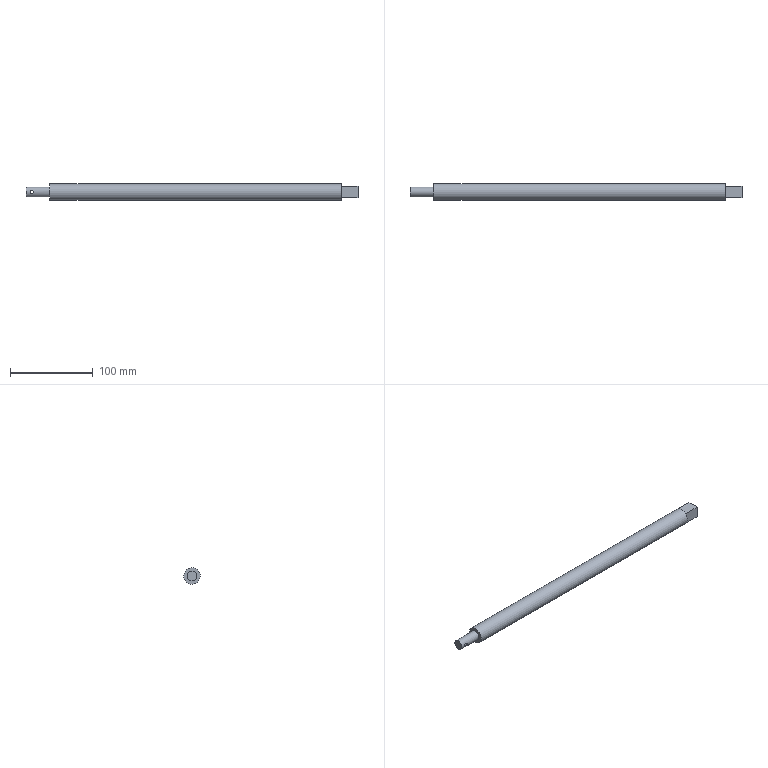Part | STEP file | SN10_001_005_FUSO | 1 solid | 11 faces | box 402 x 20 x 20 mm | volume 117949 mm3 | plane 8 | cylinder 3 | commonest cylinder face diameters 4 x1 12 x1 20 x1
STEP:
#1=CARTESIAN_POINT('',(0.,0.,0.));
#2=DIRECTION('',(0.,0.,1.));
#3=DIRECTION('',(1.,0.,0.));
#4=AXIS2_PLACEMENT_3D('',#1,#2,#3);
#5=CARTESIAN_POINT('',(67.,216.956,-8.776));
#6=VERTEX_POINT('',#5);
#7=CARTESIAN_POINT('',(67.,221.75,0.));
#8=DIRECTION('',(-1.,0.,0.));
#9=DIRECTION('',(0.,1.,0.));
#10=AXIS2_PLACEMENT_3D('',#7,#8,#9);
#11=CIRCLE('',#10,10.);
#12=CARTESIAN_POINT('',(239.,221.75,0.));
#13=DIRECTION('',(-1.,0.,0.));
#14=DIRECTION('',(0.,0.4794,0.8776));
#15=AXIS2_PLACEMENT_3D('',#12,#13,#14);
#16=CYLINDRICAL_SURFACE('',#15,10.);
#17=CARTESIAN_POINT('',(1.071,172.));
#18=DIRECTION('',(1.,0.));
#19=VECTOR('',#18,1.);
#20=LINE('',#17,#19);
#21=(GEOMETRIC_REPRESENTATION_CONTEXT(2)PARAMETRIC_REPRESENTATION_CONTEXT()REPRESENTATION_CONTEXT('',''));
#22=DEFINITIONAL_REPRESENTATION('',(#20),#21);
#23=PCURVE('',#16,#22);
#24=CARTESIAN_POINT('',(67.,221.75,6.));
#25=DIRECTION('',(-1.,0.,0.));
#26=DIRECTION('',(0.,0.,1.));
#27=AXIS2_PLACEMENT_3D('',#24,#25,#26);
#28=PLANE('',#27);
#29=CARTESIAN_POINT('',(-6.,0.));
#30=DIRECTION('',(0.,1.));
#31=AXIS2_PLACEMENT_2D('',#29,#30);
#32=CIRCLE('',#31,10.);
#33=(GEOMETRIC_REPRESENTATION_CONTEXT(2)PARAMETRIC_REPRESENTATION_CONTEXT()REPRESENTATION_CONTEXT('',''));
#34=DEFINITIONAL_REPRESENTATION('',(#32),#33);
#35=PCURVE('',#28,#34);
#36=SURFACE_CURVE('',#11,(#23,#35),.PCURVE_S1.);
#37=EDGE_CURVE('',#6,#6,#36,.T.);
#38=ORIENTED_EDGE('',*,*,#37,.F.);
#39=CARTESIAN_POINT('',(420.,216.956,-8.776));
#40=VERTEX_POINT('',#39);
#41=CARTESIAN_POINT('',(420.,216.956,-8.776));
#42=CARTESIAN_POINT('',(67.,216.956,-8.776));
#43=B_SPLINE_CURVE_WITH_KNOTS('',1,(#41,#42),.UNSPECIFIED.,.F.,.F.,(2,2),(-181.,172.),.PIECEWISE_BEZIER_KNOTS.);
#44=CARTESIAN_POINT('',(3.142,0.));
#45=DIRECTION('',(0.,1.));
#46=VECTOR('',#45,1.);
#47=LINE('',#44,#46);
#48=(GEOMETRIC_REPRESENTATION_CONTEXT(2)PARAMETRIC_REPRESENTATION_CONTEXT()REPRESENTATION_CONTEXT('',''));
#49=DEFINITIONAL_REPRESENTATION('',(#47),#48);
#50=PCURVE('',#16,#49);
#51=CARTESIAN_POINT('',(9.425,0.));
#52=DIRECTION('',(0.,1.));
#53=VECTOR('',#52,1.);
#54=LINE('',#51,#53);
#55=(GEOMETRIC_REPRESENTATION_CONTEXT(2)PARAMETRIC_REPRESENTATION_CONTEXT()REPRESENTATION_CONTEXT('',''));
#56=DEFINITIONAL_REPRESENTATION('',(#54),#55);
#57=PCURVE('',#16,#56);
#58=SEAM_CURVE('',#43,(#50,#57),.PCURVE_S1.);
#59=EDGE_CURVE('',#40,#6,#58,.T.);
#60=ORIENTED_EDGE('',*,*,#59,.F.);
#61=CARTESIAN_POINT('',(420.,221.75,0.));
#62=DIRECTION('',(-1.,0.,0.));
#63=DIRECTION('',(0.,1.,0.));
#64=AXIS2_PLACEMENT_3D('',#61,#62,#63);
#65=CIRCLE('',#64,10.);
#66=CARTESIAN_POINT('',(1.071,-181.));
#67=DIRECTION('',(1.,0.));
#68=VECTOR('',#67,1.);
#69=LINE('',#66,#68);
#70=(GEOMETRIC_REPRESENTATION_CONTEXT(2)PARAMETRIC_REPRESENTATION_CONTEXT()REPRESENTATION_CONTEXT('',''));
#71=DEFINITIONAL_REPRESENTATION('',(#69),#70);
#72=PCURVE('',#16,#71);
#73=CARTESIAN_POINT('',(420.,221.75,10.));
#74=DIRECTION('',(-1.,0.,0.));
#75=DIRECTION('',(0.,0.,1.));
#76=AXIS2_PLACEMENT_3D('',#73,#74,#75);
#77=PLANE('',#76);
#78=CARTESIAN_POINT('',(-10.,0.));
#79=DIRECTION('',(0.,1.));
#80=AXIS2_PLACEMENT_2D('',#78,#79);
#81=CIRCLE('',#80,10.);
#82=(GEOMETRIC_REPRESENTATION_CONTEXT(2)PARAMETRIC_REPRESENTATION_CONTEXT()REPRESENTATION_CONTEXT('',''));
#83=DEFINITIONAL_REPRESENTATION('',(#81),#82);
#84=PCURVE('',#77,#83);
#85=SURFACE_CURVE('',#65,(#72,#84),.PCURVE_S1.);
#86=EDGE_CURVE('',#40,#40,#85,.T.);
#87=ORIENTED_EDGE('',*,*,#86,.T.);
#88=ORIENTED_EDGE('',*,*,#59,.T.);
#89=EDGE_LOOP('',(#38,#60,#87,#88));
#90=FACE_BOUND('',#89,.T.);
#91=ADVANCED_FACE('',(#90),#16,.T.);
#92=CARTESIAN_POINT('',(38.,224.627,5.265));
#93=VERTEX_POINT('',#92);
#94=CARTESIAN_POINT('',(38.,221.75,0.));
#95=DIRECTION('',(-1.,0.,0.));
#96=DIRECTION('',(0.,1.,0.));
#97=AXIS2_PLACEMENT_3D('',#94,#95,#96);
#98=CIRCLE('',#97,6.);
#99=CARTESIAN_POINT('',(38.,221.75,0.));
#100=DIRECTION('',(-1.,0.,0.));
#101=DIRECTION('',(0.,0.,1.));
#102=AXIS2_PLACEMENT_3D('',#99,#100,#101);
#103=PLANE('',#102);
#104=CARTESIAN_POINT('',(0.,0.));
#105=DIRECTION('',(0.,1.));
#106=AXIS2_PLACEMENT_2D('',#104,#105);
#107=CIRCLE('',#106,6.);
#108=(GEOMETRIC_REPRESENTATION_CONTEXT(2)PARAMETRIC_REPRESENTATION_CONTEXT()REPRESENTATION_CONTEXT('',''));
#109=DEFINITIONAL_REPRESENTATION('',(#107),#108);
#110=PCURVE('',#103,#109);
#111=CARTESIAN_POINT('',(239.,221.75,0.));
#112=DIRECTION('',(-1.,0.,0.));
#113=DIRECTION('',(0.,0.4794,0.8776));
#114=AXIS2_PLACEMENT_3D('',#111,#112,#113);
#115=CYLINDRICAL_SURFACE('',#114,6.);
#116=CARTESIAN_POINT('',(-5.212,201.));
#117=DIRECTION('',(1.,0.));
#118=VECTOR('',#117,1.);
#119=LINE('',#116,#118);
#120=(GEOMETRIC_REPRESENTATION_CONTEXT(2)PARAMETRIC_REPRESENTATION_CONTEXT()REPRESENTATION_CONTEXT('',''));
#121=DEFINITIONAL_REPRESENTATION('',(#119),#120);
#122=PCURVE('',#115,#121);
#123=SURFACE_CURVE('',#98,(#110,#122),.PCURVE_S1.);
#124=EDGE_CURVE('',#93,#93,#123,.T.);
#125=ORIENTED_EDGE('',*,*,#124,.T.);
#126=EDGE_LOOP('',(#125));
#127=FACE_BOUND('',#126,.T.);
#128=ADVANCED_FACE('',(#127),#103,.T.);
#129=ORIENTED_EDGE('',*,*,#37,.T.);
#130=EDGE_LOOP('',(#129));
#131=FACE_BOUND('',#130,.T.);
#132=CARTESIAN_POINT('',(67.,224.627,5.265));
#133=VERTEX_POINT('',#132);
#134=CARTESIAN_POINT('',(67.,221.75,0.));
#135=DIRECTION('',(-1.,0.,0.));
#136=DIRECTION('',(0.,1.,0.));
#137=AXIS2_PLACEMENT_3D('',#134,#135,#136);
#138=CIRCLE('',#137,6.);
#139=CARTESIAN_POINT('',(-6.,0.));
#140=DIRECTION('',(0.,1.));
#141=AXIS2_PLACEMENT_2D('',#139,#140);
#142=CIRCLE('',#141,6.);
#143=(GEOMETRIC_REPRESENTATION_CONTEXT(2)PARAMETRIC_REPRESENTATION_CONTEXT()REPRESENTATION_CONTEXT('',''));
#144=DEFINITIONAL_REPRESENTATION('',(#142),#143);
#145=PCURVE('',#28,#144);
#146=CARTESIAN_POINT('',(-5.212,172.));
#147=DIRECTION('',(1.,0.));
#148=VECTOR('',#147,1.);
#149=LINE('',#146,#148);
#150=(GEOMETRIC_REPRESENTATION_CONTEXT(2)PARAMETRIC_REPRESENTATION_CONTEXT()REPRESENTATION_CONTEXT('',''));
#151=DEFINITIONAL_REPRESENTATION('',(#149),#150);
#152=PCURVE('',#115,#151);
#153=SURFACE_CURVE('',#138,(#145,#152),.PCURVE_S1.);
#154=EDGE_CURVE('',#133,#133,#153,.T.);
#155=ORIENTED_EDGE('',*,*,#154,.F.);
#156=EDGE_LOOP('',(#155));
#157=FACE_BOUND('',#156,.T.);
#158=ADVANCED_FACE('',(#131,#157),#28,.T.);
#159=ORIENTED_EDGE('',*,*,#124,.F.);
#160=CARTESIAN_POINT('',(67.,224.627,5.265));
#161=CARTESIAN_POINT('',(38.,224.627,5.265));
#162=B_SPLINE_CURVE_WITH_KNOTS('',1,(#160,#161),.UNSPECIFIED.,.F.,.F.,(2,2),(172.,201.),.PIECEWISE_BEZIER_KNOTS.);
#163=CARTESIAN_POINT('',(0.,0.));
#164=DIRECTION('',(0.,1.));
#165=VECTOR('',#164,1.);
#166=LINE('',#163,#165);
#167=(GEOMETRIC_REPRESENTATION_CONTEXT(2)PARAMETRIC_REPRESENTATION_CONTEXT()REPRESENTATION_CONTEXT('',''));
#168=DEFINITIONAL_REPRESENTATION('',(#166),#167);
#169=PCURVE('',#115,#168);
#170=CARTESIAN_POINT('',(6.283,0.));
#171=DIRECTION('',(0.,1.));
#172=VECTOR('',#171,1.);
#173=LINE('',#170,#172);
#174=(GEOMETRIC_REPRESENTATION_CONTEXT(2)PARAMETRIC_REPRESENTATION_CONTEXT()REPRESENTATION_CONTEXT('',''));
#175=DEFINITIONAL_REPRESENTATION('',(#173),#174);
#176=PCURVE('',#115,#175);
#177=SEAM_CURVE('',#162,(#169,#176),.PCURVE_S1.);
#178=EDGE_CURVE('',#133,#93,#177,.T.);
#179=ORIENTED_EDGE('',*,*,#178,.F.);
#180=ORIENTED_EDGE('',*,*,#154,.T.);
#181=ORIENTED_EDGE('',*,*,#178,.T.);
#182=EDGE_LOOP('',(#159,#179,#180,#181));
#183=FACE_BOUND('',#182,.T.);
#184=CARTESIAN_POINT('',(45.,227.407,2.));
#185=VERTEX_POINT('',#184);
#186=CARTESIAN_POINT('',(45.,227.407,-2.));
#187=VERTEX_POINT('',#186);
#188=CARTESIAN_POINT('',(45.,227.407,2.));
#189=CARTESIAN_POINT('',(45.253,227.407,2.));
#190=CARTESIAN_POINT('',(45.522,227.426,1.949));
#191=CARTESIAN_POINT('',(46.014,227.492,1.744));
#192=CARTESIAN_POINT('',(46.238,227.538,1.591));
#193=CARTESIAN_POINT('',(46.591,227.624,1.238));
#194=CARTESIAN_POINT('',(46.744,227.669,1.014));
#195=CARTESIAN_POINT('',(46.949,227.732,0.5219));
#196=CARTESIAN_POINT('',(47.,227.75,0.2532));
#197=CARTESIAN_POINT('',(47.,227.75,-0.2532));
#198=CARTESIAN_POINT('',(46.949,227.732,-0.5219));
#199=CARTESIAN_POINT('',(46.744,227.669,-1.014));
#200=CARTESIAN_POINT('',(46.591,227.624,-1.238));
#201=CARTESIAN_POINT('',(46.238,227.538,-1.591));
#202=CARTESIAN_POINT('',(46.014,227.492,-1.744));
#203=CARTESIAN_POINT('',(45.522,227.426,-1.949));
#204=CARTESIAN_POINT('',(45.253,227.407,-2.));
#205=CARTESIAN_POINT('',(45.,227.407,-2.));
#206=B_SPLINE_CURVE_WITH_KNOTS('',3,(#188,#189,#190,#191,#192,#193,#194,#195,#196,#197,#198,#199,#200,#201,#202,#203,#204,#205),.UNSPECIFIED.,.F.,.F.,(4,2,2,2,2,2,2,2,4),(0.6078,0.6837,0.7597,0.8357,0.9116,0.9876,1.064,1.14,1.216),.UNSPECIFIED.);
#207=CARTESIAN_POINT('',(0.731,194.));
#208=CARTESIAN_POINT('',(0.731,193.954));
#209=CARTESIAN_POINT('',(0.7316,193.861));
#210=CARTESIAN_POINT('',(0.7342,193.72));
#211=CARTESIAN_POINT('',(0.7387,193.578));
#212=CARTESIAN_POINT('',(0.745,193.437));
#213=CARTESIAN_POINT('',(0.753,193.299));
#214=CARTESIAN_POINT('',(0.7628,193.165));
#215=CARTESIAN_POINT('',(0.7742,193.035));
#216=CARTESIAN_POINT('',(0.7871,192.912));
#217=CARTESIAN_POINT('',(0.8013,192.795));
#218=CARTESIAN_POINT('',(0.8166,192.685));
#219=CARTESIAN_POINT('',(0.8326,192.585));
#220=CARTESIAN_POINT('',(0.8498,192.491));
#221=CARTESIAN_POINT('',(0.8685,192.403));
#222=CARTESIAN_POINT('',(0.8883,192.321));
#223=CARTESIAN_POINT('',(0.9093,192.247));
#224=CARTESIAN_POINT('',(0.9311,192.181));
#225=CARTESIAN_POINT('',(0.9537,192.125));
#226=CARTESIAN_POINT('',(0.9768,192.079));
#227=CARTESIAN_POINT('',(1.,192.044));
#228=CARTESIAN_POINT('',(1.024,192.019));
#229=CARTESIAN_POINT('',(1.048,192.003));
#230=CARTESIAN_POINT('',(1.071,191.998));
#231=CARTESIAN_POINT('',(1.094,192.003));
#232=CARTESIAN_POINT('',(1.118,192.019));
#233=CARTESIAN_POINT('',(1.141,192.044));
#234=CARTESIAN_POINT('',(1.165,192.079));
#235=CARTESIAN_POINT('',(1.188,192.125));
#236=CARTESIAN_POINT('',(1.211,192.181));
#237=CARTESIAN_POINT('',(1.232,192.247));
#238=CARTESIAN_POINT('',(1.253,192.321));
#239=CARTESIAN_POINT('',(1.273,192.403));
#240=CARTESIAN_POINT('',(1.292,192.491));
#241=CARTESIAN_POINT('',(1.309,192.585));
#242=CARTESIAN_POINT('',(1.325,192.685));
#243=CARTESIAN_POINT('',(1.34,192.795));
#244=CARTESIAN_POINT('',(1.354,192.912));
#245=CARTESIAN_POINT('',(1.367,193.035));
#246=CARTESIAN_POINT('',(1.379,193.165));
#247=CARTESIAN_POINT('',(1.389,193.299));
#248=CARTESIAN_POINT('',(1.397,193.437));
#249=CARTESIAN_POINT('',(1.403,193.578));
#250=CARTESIAN_POINT('',(1.407,193.72));
#251=CARTESIAN_POINT('',(1.41,193.861));
#252=CARTESIAN_POINT('',(1.411,193.954));
#253=CARTESIAN_POINT('',(1.411,194.));
#254=B_SPLINE_CURVE_WITH_KNOTS('',3,(#207,#208,#209,#210,#211,#212,#213,#214,#215,#216,#217,#218,#219,#220,#221,#222,#223,#224,#225,#226,#227,#228,#229,#230,#231,#232,#233,#234,#235,#236,#237,#238,#239,#240,#241,#242,#243,#244,#245,#246,#247,#248,#249,#250,#251,#252,#253),.UNSPECIFIED.,.F.,.F.,(4,1,1,1,1,1,1,1,1,1,1,1,1,1,1,1,1,1,1,1,1,1,1,1,1,1,1,1,1,1,1,1,1,1,1,1,1,1,1,1,1,1,1,1,4),(0.6078,0.6216,0.6354,0.6492,0.663,0.6768,0.6906,0.7044,0.7183,0.7321,0.7459,0.7597,0.7735,0.7873,0.8011,0.815,0.8288,0.8426,0.8564,0.8702,0.884,0.8978,0.9116,0.9255,0.9393,0.9531,0.9669,0.9807,0.9945,1.008,1.022,1.036,1.05,1.064,1.077,1.091,1.105,1.119,1.133,1.146,1.16,1.174,1.188,1.202,1.216),.QUASI_UNIFORM_KNOTS.);
#255=(GEOMETRIC_REPRESENTATION_CONTEXT(2)PARAMETRIC_REPRESENTATION_CONTEXT()REPRESENTATION_CONTEXT('',''));
#256=DEFINITIONAL_REPRESENTATION('',(#254),#255);
#257=PCURVE('',#115,#256);
#258=CARTESIAN_POINT('',(45.,221.75,0.));
#259=DIRECTION('',(0.,1.,0.));
#260=DIRECTION('',(0.,0.,1.));
#261=AXIS2_PLACEMENT_3D('',#258,#259,#260);
#262=CYLINDRICAL_SURFACE('',#261,2.);
#263=CARTESIAN_POINT('',(0.,5.657));
#264=CARTESIAN_POINT('',(0.02302,5.657));
#265=CARTESIAN_POINT('',(0.06957,5.658));
#266=CARTESIAN_POINT('',(0.1406,5.664));
#267=CARTESIAN_POINT('',(0.2125,5.672));
#268=CARTESIAN_POINT('',(0.285,5.684));
#269=CARTESIAN_POINT('',(0.3577,5.7));
#270=CARTESIAN_POINT('',(0.4304,5.718));
#271=CARTESIAN_POINT('',(0.5029,5.738));
#272=CARTESIAN_POINT('',(0.575,5.76));
#273=CARTESIAN_POINT('',(0.6463,5.784));
#274=CARTESIAN_POINT('',(0.7167,5.807));
#275=CARTESIAN_POINT('',(0.7852,5.831));
#276=CARTESIAN_POINT('',(0.8538,5.854));
#277=CARTESIAN_POINT('',(0.9242,5.878));
#278=CARTESIAN_POINT('',(0.9955,5.901));
#279=CARTESIAN_POINT('',(1.068,5.922));
#280=CARTESIAN_POINT('',(1.14,5.942));
#281=CARTESIAN_POINT('',(1.213,5.959));
#282=CARTESIAN_POINT('',(1.286,5.974));
#283=CARTESIAN_POINT('',(1.358,5.985));
#284=CARTESIAN_POINT('',(1.43,5.994));
#285=CARTESIAN_POINT('',(1.501,5.999));
#286=CARTESIAN_POINT('',(1.571,6.001));
#287=CARTESIAN_POINT('',(1.64,5.999));
#288=CARTESIAN_POINT('',(1.711,5.994));
#289=CARTESIAN_POINT('',(1.783,5.985));
#290=CARTESIAN_POINT('',(1.856,5.974));
#291=CARTESIAN_POINT('',(1.929,5.959));
#292=CARTESIAN_POINT('',(2.001,5.942));
#293=CARTESIAN_POINT('',(2.074,5.922));
#294=CARTESIAN_POINT('',(2.146,5.901));
#295=CARTESIAN_POINT('',(2.217,5.878));
#296=CARTESIAN_POINT('',(2.288,5.854));
#297=CARTESIAN_POINT('',(2.356,5.831));
#298=CARTESIAN_POINT('',(2.425,5.807));
#299=CARTESIAN_POINT('',(2.495,5.784));
#300=CARTESIAN_POINT('',(2.567,5.76));
#301=CARTESIAN_POINT('',(2.639,5.738));
#302=CARTESIAN_POINT('',(2.711,5.718));
#303=CARTESIAN_POINT('',(2.784,5.7));
#304=CARTESIAN_POINT('',(2.857,5.684));
#305=CARTESIAN_POINT('',(2.929,5.672));
#306=CARTESIAN_POINT('',(3.001,5.664));
#307=CARTESIAN_POINT('',(3.072,5.658));
#308=CARTESIAN_POINT('',(3.119,5.657));
#309=CARTESIAN_POINT('',(3.142,5.657));
#310=B_SPLINE_CURVE_WITH_KNOTS('',3,(#263,#264,#265,#266,#267,#268,#269,#270,#271,#272,#273,#274,#275,#276,#277,#278,#279,#280,#281,#282,#283,#284,#285,#286,#287,#288,#289,#290,#291,#292,#293,#294,#295,#296,#297,#298,#299,#300,#301,#302,#303,#304,#305,#306,#307,#308,#309),.UNSPECIFIED.,.F.,.F.,(4,1,1,1,1,1,1,1,1,1,1,1,1,1,1,1,1,1,1,1,1,1,1,1,1,1,1,1,1,1,1,1,1,1,1,1,1,1,1,1,1,1,1,1,4),(0.6078,0.6216,0.6354,0.6492,0.663,0.6768,0.6906,0.7044,0.7183,0.7321,0.7459,0.7597,0.7735,0.7873,0.8011,0.815,0.8288,0.8426,0.8564,0.8702,0.884,0.8978,0.9116,0.9255,0.9393,0.9531,0.9669,0.9807,0.9945,1.008,1.022,1.036,1.05,1.064,1.077,1.091,1.105,1.119,1.133,1.146,1.16,1.174,1.188,1.202,1.216),.QUASI_UNIFORM_KNOTS.);
#311=(GEOMETRIC_REPRESENTATION_CONTEXT(2)PARAMETRIC_REPRESENTATION_CONTEXT()REPRESENTATION_CONTEXT('',''));
#312=DEFINITIONAL_REPRESENTATION('',(#310),#311);
#313=PCURVE('',#262,#312);
#314=SURFACE_CURVE('',#206,(#257,#313),.PCURVE_S1.);
#315=EDGE_CURVE('',#185,#187,#314,.T.);
#316=ORIENTED_EDGE('',*,*,#315,.F.);
#317=CARTESIAN_POINT('',(45.,227.407,-2.));
#318=CARTESIAN_POINT('',(44.747,227.407,-2.));
#319=CARTESIAN_POINT('',(44.478,227.426,-1.949));
#320=CARTESIAN_POINT('',(43.986,227.492,-1.744));
#321=CARTESIAN_POINT('',(43.762,227.538,-1.591));
#322=CARTESIAN_POINT('',(43.409,227.624,-1.238));
#323=CARTESIAN_POINT('',(43.256,227.669,-1.014));
#324=CARTESIAN_POINT('',(43.051,227.732,-0.5219));
#325=CARTESIAN_POINT('',(43.,227.75,-0.2532));
#326=CARTESIAN_POINT('',(43.,227.75,0.2532));
#327=CARTESIAN_POINT('',(43.051,227.732,0.5219));
#328=CARTESIAN_POINT('',(43.256,227.669,1.014));
#329=CARTESIAN_POINT('',(43.409,227.624,1.238));
#330=CARTESIAN_POINT('',(43.762,227.538,1.591));
#331=CARTESIAN_POINT('',(43.986,227.492,1.744));
#332=CARTESIAN_POINT('',(44.478,227.426,1.949));
#333=CARTESIAN_POINT('',(44.747,227.407,2.));
#334=CARTESIAN_POINT('',(45.,227.407,2.));
#335=B_SPLINE_CURVE_WITH_KNOTS('',3,(#317,#318,#319,#320,#321,#322,#323,#324,#325,#326,#327,#328,#329,#330,#331,#332,#333,#334),.UNSPECIFIED.,.F.,.F.,(4,2,2,2,2,2,2,2,4),(0.,0.07599,0.152,0.2279,0.3039,0.3798,0.4558,0.5318,0.6078),.UNSPECIFIED.);
#336=CARTESIAN_POINT('',(1.411,194.));
#337=CARTESIAN_POINT('',(1.411,194.046));
#338=CARTESIAN_POINT('',(1.41,194.139));
#339=CARTESIAN_POINT('',(1.407,194.28));
#340=CARTESIAN_POINT('',(1.403,194.422));
#341=CARTESIAN_POINT('',(1.397,194.563));
#342=CARTESIAN_POINT('',(1.389,194.701));
#343=CARTESIAN_POINT('',(1.379,194.835));
#344=CARTESIAN_POINT('',(1.367,194.965));
#345=CARTESIAN_POINT('',(1.354,195.088));
#346=CARTESIAN_POINT('',(1.34,195.205));
#347=CARTESIAN_POINT('',(1.325,195.315));
#348=CARTESIAN_POINT('',(1.309,195.415));
#349=CARTESIAN_POINT('',(1.292,195.509));
#350=CARTESIAN_POINT('',(1.273,195.597));
#351=CARTESIAN_POINT('',(1.253,195.679));
#352=CARTESIAN_POINT('',(1.232,195.753));
#353=CARTESIAN_POINT('',(1.211,195.819));
#354=CARTESIAN_POINT('',(1.188,195.875));
#355=CARTESIAN_POINT('',(1.165,195.921));
#356=CARTESIAN_POINT('',(1.141,195.956));
#357=CARTESIAN_POINT('',(1.118,195.981));
#358=CARTESIAN_POINT('',(1.094,195.997));
#359=CARTESIAN_POINT('',(1.071,196.002));
#360=CARTESIAN_POINT('',(1.048,195.997));
#361=CARTESIAN_POINT('',(1.024,195.981));
#362=CARTESIAN_POINT('',(1.,195.956));
#363=CARTESIAN_POINT('',(0.9768,195.921));
#364=CARTESIAN_POINT('',(0.9537,195.875));
#365=CARTESIAN_POINT('',(0.9311,195.819));
#366=CARTESIAN_POINT('',(0.9093,195.753));
#367=CARTESIAN_POINT('',(0.8883,195.679));
#368=CARTESIAN_POINT('',(0.8685,195.597));
#369=CARTESIAN_POINT('',(0.8498,195.509));
#370=CARTESIAN_POINT('',(0.8326,195.415));
#371=CARTESIAN_POINT('',(0.8166,195.315));
#372=CARTESIAN_POINT('',(0.8013,195.205));
#373=CARTESIAN_POINT('',(0.7871,195.088));
#374=CARTESIAN_POINT('',(0.7742,194.965));
#375=CARTESIAN_POINT('',(0.7628,194.835));
#376=CARTESIAN_POINT('',(0.753,194.701));
#377=CARTESIAN_POINT('',(0.745,194.563));
#378=CARTESIAN_POINT('',(0.7387,194.422));
#379=CARTESIAN_POINT('',(0.7342,194.28));
#380=CARTESIAN_POINT('',(0.7316,194.139));
#381=CARTESIAN_POINT('',(0.731,194.046));
#382=CARTESIAN_POINT('',(0.731,194.));
#383=B_SPLINE_CURVE_WITH_KNOTS('',3,(#336,#337,#338,#339,#340,#341,#342,#343,#344,#345,#346,#347,#348,#349,#350,#351,#352,#353,#354,#355,#356,#357,#358,#359,#360,#361,#362,#363,#364,#365,#366,#367,#368,#369,#370,#371,#372,#373,#374,#375,#376,#377,#378,#379,#380,#381,#382),.UNSPECIFIED.,.F.,.F.,(4,1,1,1,1,1,1,1,1,1,1,1,1,1,1,1,1,1,1,1,1,1,1,1,1,1,1,1,1,1,1,1,1,1,1,1,1,1,1,1,1,1,1,1,4),(0.,0.01381,0.02763,0.04144,0.05525,0.06906,0.08288,0.09669,0.1105,0.1243,0.1381,0.1519,0.1658,0.1796,0.1934,0.2072,0.221,0.2348,0.2486,0.2624,0.2763,0.2901,0.3039,0.3177,0.3315,0.3453,0.3591,0.3729,0.3868,0.4006,0.4144,0.4282,0.442,0.4558,0.4696,0.4834,0.4973,0.5111,0.5249,0.5387,0.5525,0.5663,0.5801,0.5939,0.6078),.QUASI_UNIFORM_KNOTS.);
#384=(GEOMETRIC_REPRESENTATION_CONTEXT(2)PARAMETRIC_REPRESENTATION_CONTEXT()REPRESENTATION_CONTEXT('',''));
#385=DEFINITIONAL_REPRESENTATION('',(#383),#384);
#386=PCURVE('',#115,#385);
#387=CARTESIAN_POINT('',(3.142,5.657));
#388=CARTESIAN_POINT('',(3.165,5.657));
#389=CARTESIAN_POINT('',(3.211,5.658));
#390=CARTESIAN_POINT('',(3.282,5.664));
#391=CARTESIAN_POINT('',(3.354,5.672));
#392=CARTESIAN_POINT('',(3.427,5.684));
#393=CARTESIAN_POINT('',(3.499,5.7));
#394=CARTESIAN_POINT('',(3.572,5.718));
#395=CARTESIAN_POINT('',(3.644,5.738));
#396=CARTESIAN_POINT('',(3.717,5.76));
#397=CARTESIAN_POINT('',(3.788,5.784));
#398=CARTESIAN_POINT('',(3.858,5.807));
#399=CARTESIAN_POINT('',(3.927,5.831));
#400=CARTESIAN_POINT('',(3.995,5.854));
#401=CARTESIAN_POINT('',(4.066,5.878));
#402=CARTESIAN_POINT('',(4.137,5.901));
#403=CARTESIAN_POINT('',(4.209,5.922));
#404=CARTESIAN_POINT('',(4.282,5.942));
#405=CARTESIAN_POINT('',(4.355,5.959));
#406=CARTESIAN_POINT('',(4.427,5.974));
#407=CARTESIAN_POINT('',(4.5,5.985));
#408=CARTESIAN_POINT('',(4.572,5.994));
#409=CARTESIAN_POINT('',(4.643,5.999));
#410=CARTESIAN_POINT('',(4.712,6.001));
#411=CARTESIAN_POINT('',(4.782,5.999));
#412=CARTESIAN_POINT('',(4.853,5.994));
#413=CARTESIAN_POINT('',(4.925,5.985));
#414=CARTESIAN_POINT('',(4.998,5.974));
#415=CARTESIAN_POINT('',(5.07,5.959));
#416=CARTESIAN_POINT('',(5.143,5.942));
#417=CARTESIAN_POINT('',(5.216,5.922));
#418=CARTESIAN_POINT('',(5.288,5.901));
#419=CARTESIAN_POINT('',(5.359,5.878));
#420=CARTESIAN_POINT('',(5.429,5.854));
#421=CARTESIAN_POINT('',(5.498,5.831));
#422=CARTESIAN_POINT('',(5.567,5.807));
#423=CARTESIAN_POINT('',(5.637,5.784));
#424=CARTESIAN_POINT('',(5.708,5.76));
#425=CARTESIAN_POINT('',(5.78,5.738));
#426=CARTESIAN_POINT('',(5.853,5.718));
#427=CARTESIAN_POINT('',(5.925,5.7));
#428=CARTESIAN_POINT('',(5.998,5.684));
#429=CARTESIAN_POINT('',(6.071,5.672));
#430=CARTESIAN_POINT('',(6.143,5.664));
#431=CARTESIAN_POINT('',(6.214,5.658));
#432=CARTESIAN_POINT('',(6.26,5.657));
#433=CARTESIAN_POINT('',(6.283,5.657));
#434=B_SPLINE_CURVE_WITH_KNOTS('',3,(#387,#388,#389,#390,#391,#392,#393,#394,#395,#396,#397,#398,#399,#400,#401,#402,#403,#404,#405,#406,#407,#408,#409,#410,#411,#412,#413,#414,#415,#416,#417,#418,#419,#420,#421,#422,#423,#424,#425,#426,#427,#428,#429,#430,#431,#432,#433),.UNSPECIFIED.,.F.,.F.,(4,1,1,1,1,1,1,1,1,1,1,1,1,1,1,1,1,1,1,1,1,1,1,1,1,1,1,1,1,1,1,1,1,1,1,1,1,1,1,1,1,1,1,1,4),(0.,0.01381,0.02763,0.04144,0.05525,0.06906,0.08288,0.09669,0.1105,0.1243,0.1381,0.1519,0.1658,0.1796,0.1934,0.2072,0.221,0.2348,0.2486,0.2624,0.2763,0.2901,0.3039,0.3177,0.3315,0.3453,0.3591,0.3729,0.3868,0.4006,0.4144,0.4282,0.442,0.4558,0.4696,0.4834,0.4973,0.5111,0.5249,0.5387,0.5525,0.5663,0.5801,0.5939,0.6078),.QUASI_UNIFORM_KNOTS.);
#435=(GEOMETRIC_REPRESENTATION_CONTEXT(2)PARAMETRIC_REPRESENTATION_CONTEXT()REPRESENTATION_CONTEXT('',''));
#436=DEFINITIONAL_REPRESENTATION('',(#434),#435);
#437=PCURVE('',#262,#436);
#438=SURFACE_CURVE('',#335,(#386,#437),.PCURVE_S1.);
#439=EDGE_CURVE('',#187,#185,#438,.T.);
#440=ORIENTED_EDGE('',*,*,#439,.F.);
#441=EDGE_LOOP('',(#316,#440));
#442=FACE_BOUND('',#441,.T.);
#443=CARTESIAN_POINT('',(45.,216.093,-2.));
#444=VERTEX_POINT('',#443);
#445=CARTESIAN_POINT('',(45.,216.093,2.));
#446=VERTEX_POINT('',#445);
#447=CARTESIAN_POINT('',(45.,216.093,-2.));
#448=CARTESIAN_POINT('',(44.747,216.093,-2.));
#449=CARTESIAN_POINT('',(44.478,216.074,-1.949));
#450=CARTESIAN_POINT('',(43.986,216.008,-1.744));
#451=CARTESIAN_POINT('',(43.762,215.962,-1.591));
#452=CARTESIAN_POINT('',(43.409,215.876,-1.238));
#453=CARTESIAN_POINT('',(43.256,215.831,-1.014));
#454=CARTESIAN_POINT('',(43.051,215.768,-0.5219));
#455=CARTESIAN_POINT('',(43.,215.75,-0.2532));
#456=CARTESIAN_POINT('',(43.,215.75,0.2532));
#457=CARTESIAN_POINT('',(43.051,215.768,0.5219));
#458=CARTESIAN_POINT('',(43.256,215.831,1.014));
#459=CARTESIAN_POINT('',(43.409,215.876,1.238));
#460=CARTESIAN_POINT('',(43.762,215.962,1.591));
#461=CARTESIAN_POINT('',(43.986,216.008,1.744));
#462=CARTESIAN_POINT('',(44.478,216.074,1.949));
#463=CARTESIAN_POINT('',(44.747,216.093,2.));
#464=CARTESIAN_POINT('',(45.,216.093,2.));
#465=B_SPLINE_CURVE_WITH_KNOTS('',3,(#447,#448,#449,#450,#451,#452,#453,#454,#455,#456,#457,#458,#459,#460,#461,#462,#463,#464),.UNSPECIFIED.,.F.,.F.,(4,2,2,2,2,2,2,2,4),(-1.216,-1.14,-1.064,-0.9876,-0.9116,-0.8357,-0.7597,-0.6837,-0.6078),.UNSPECIFIED.);
#466=CARTESIAN_POINT('',(3.873,194.));
#467=CARTESIAN_POINT('',(3.873,194.046));
#468=CARTESIAN_POINT('',(3.873,194.139));
#469=CARTESIAN_POINT('',(3.876,194.28));
#470=CARTESIAN_POINT('',(3.88,194.422));
#471=CARTESIAN_POINT('',(3.887,194.563));
#472=CARTESIAN_POINT('',(3.895,194.701));
#473=CARTESIAN_POINT('',(3.904,194.835));
#474=CARTESIAN_POINT('',(3.916,194.965));
#475=CARTESIAN_POINT('',(3.929,195.088));
#476=CARTESIAN_POINT('',(3.943,195.205));
#477=CARTESIAN_POINT('',(3.958,195.315));
#478=CARTESIAN_POINT('',(3.974,195.415));
#479=CARTESIAN_POINT('',(3.991,195.509));
#480=CARTESIAN_POINT('',(4.01,195.597));
#481=CARTESIAN_POINT('',(4.03,195.679));
#482=CARTESIAN_POINT('',(4.051,195.753));
#483=CARTESIAN_POINT('',(4.073,195.819));
#484=CARTESIAN_POINT('',(4.095,195.875));
#485=CARTESIAN_POINT('',(4.118,195.921));
#486=CARTESIAN_POINT('',(4.142,195.956));
#487=CARTESIAN_POINT('',(4.166,195.981));
#488=CARTESIAN_POINT('',(4.189,195.997));
#489=CARTESIAN_POINT('',(4.212,196.002));
#490=CARTESIAN_POINT('',(4.236,195.997));
#491=CARTESIAN_POINT('',(4.259,195.981));
#492=CARTESIAN_POINT('',(4.283,195.956));
#493=CARTESIAN_POINT('',(4.306,195.921));
#494=CARTESIAN_POINT('',(4.33,195.875));
#495=CARTESIAN_POINT('',(4.352,195.819));
#496=CARTESIAN_POINT('',(4.374,195.753));
#497=CARTESIAN_POINT('',(4.395,195.679));
#498=CARTESIAN_POINT('',(4.415,195.597));
#499=CARTESIAN_POINT('',(4.433,195.509));
#500=CARTESIAN_POINT('',(4.451,195.415));
#501=CARTESIAN_POINT('',(4.467,195.315));
#502=CARTESIAN_POINT('',(4.482,195.205));
#503=CARTESIAN_POINT('',(4.496,195.088));
#504=CARTESIAN_POINT('',(4.509,194.965));
#505=CARTESIAN_POINT('',(4.52,194.835));
#506=CARTESIAN_POINT('',(4.53,194.701));
#507=CARTESIAN_POINT('',(4.538,194.563));
#508=CARTESIAN_POINT('',(4.544,194.422));
#509=CARTESIAN_POINT('',(4.549,194.28));
#510=CARTESIAN_POINT('',(4.552,194.139));
#511=CARTESIAN_POINT('',(4.552,194.046));
#512=CARTESIAN_POINT('',(4.552,194.));
#513=B_SPLINE_CURVE_WITH_KNOTS('',3,(#466,#467,#468,#469,#470,#471,#472,#473,#474,#475,#476,#477,#478,#479,#480,#481,#482,#483,#484,#485,#486,#487,#488,#489,#490,#491,#492,#493,#494,#495,#496,#497,#498,#499,#500,#501,#502,#503,#504,#505,#506,#507,#508,#509,#510,#511,#512),.UNSPECIFIED.,.F.,.F.,(4,1,1,1,1,1,1,1,1,1,1,1,1,1,1,1,1,1,1,1,1,1,1,1,1,1,1,1,1,1,1,1,1,1,1,1,1,1,1,1,1,1,1,1,4),(-1.216,-1.202,-1.188,-1.174,-1.16,-1.146,-1.133,-1.119,-1.105,-1.091,-1.077,-1.064,-1.05,-1.036,-1.022,-1.008,-0.9945,-0.9807,-0.9669,-0.9531,-0.9393,-0.9255,-0.9116,-0.8978,-0.884,-0.8702,-0.8564,-0.8426,-0.8288,-0.815,-0.8011,-0.7873,-0.7735,-0.7597,-0.7459,-0.7321,-0.7183,-0.7044,-0.6906,-0.6768,-0.663,-0.6492,-0.6354,-0.6216,-0.6078),.QUASI_UNIFORM_KNOTS.);
#514=(GEOMETRIC_REPRESENTATION_CONTEXT(2)PARAMETRIC_REPRESENTATION_CONTEXT()REPRESENTATION_CONTEXT('',''));
#515=DEFINITIONAL_REPRESENTATION('',(#513),#514);
#516=PCURVE('',#115,#515);
#517=CARTESIAN_POINT('',(3.142,-5.657));
#518=CARTESIAN_POINT('',(3.165,-5.657));
#519=CARTESIAN_POINT('',(3.211,-5.658));
#520=CARTESIAN_POINT('',(3.282,-5.664));
#521=CARTESIAN_POINT('',(3.354,-5.672));
#522=CARTESIAN_POINT('',(3.427,-5.684));
#523=CARTESIAN_POINT('',(3.499,-5.7));
#524=CARTESIAN_POINT('',(3.572,-5.718));
#525=CARTESIAN_POINT('',(3.644,-5.738));
#526=CARTESIAN_POINT('',(3.717,-5.76));
#527=CARTESIAN_POINT('',(3.788,-5.784));
#528=CARTESIAN_POINT('',(3.858,-5.807));
#529=CARTESIAN_POINT('',(3.927,-5.831));
#530=CARTESIAN_POINT('',(3.995,-5.854));
#531=CARTESIAN_POINT('',(4.066,-5.878));
#532=CARTESIAN_POINT('',(4.137,-5.901));
#533=CARTESIAN_POINT('',(4.209,-5.922));
#534=CARTESIAN_POINT('',(4.282,-5.942));
#535=CARTESIAN_POINT('',(4.355,-5.959));
#536=CARTESIAN_POINT('',(4.427,-5.974));
#537=CARTESIAN_POINT('',(4.5,-5.985));
#538=CARTESIAN_POINT('',(4.572,-5.994));
#539=CARTESIAN_POINT('',(4.643,-5.999));
#540=CARTESIAN_POINT('',(4.712,-6.001));
#541=CARTESIAN_POINT('',(4.782,-5.999));
#542=CARTESIAN_POINT('',(4.853,-5.994));
#543=CARTESIAN_POINT('',(4.925,-5.985));
#544=CARTESIAN_POINT('',(4.998,-5.974));
#545=CARTESIAN_POINT('',(5.07,-5.959));
#546=CARTESIAN_POINT('',(5.143,-5.942));
#547=CARTESIAN_POINT('',(5.216,-5.922));
#548=CARTESIAN_POINT('',(5.288,-5.901));
#549=CARTESIAN_POINT('',(5.359,-5.878));
#550=CARTESIAN_POINT('',(5.429,-5.854));
#551=CARTESIAN_POINT('',(5.498,-5.831));
#552=CARTESIAN_POINT('',(5.567,-5.807));
#553=CARTESIAN_POINT('',(5.637,-5.784));
#554=CARTESIAN_POINT('',(5.708,-5.76));
#555=CARTESIAN_POINT('',(5.78,-5.738));
#556=CARTESIAN_POINT('',(5.853,-5.718));
#557=CARTESIAN_POINT('',(5.925,-5.7));
#558=CARTESIAN_POINT('',(5.998,-5.684));
#559=CARTESIAN_POINT('',(6.071,-5.672));
#560=CARTESIAN_POINT('',(6.143,-5.664));
#561=CARTESIAN_POINT('',(6.214,-5.658));
#562=CARTESIAN_POINT('',(6.26,-5.657));
#563=CARTESIAN_POINT('',(6.283,-5.657));
#564=B_SPLINE_CURVE_WITH_KNOTS('',3,(#517,#518,#519,#520,#521,#522,#523,#524,#525,#526,#527,#528,#529,#530,#531,#532,#533,#534,#535,#536,#537,#538,#539,#540,#541,#542,#543,#544,#545,#546,#547,#548,#549,#550,#551,#552,#553,#554,#555,#556,#557,#558,#559,#560,#561,#562,#563),.UNSPECIFIED.,.F.,.F.,(4,1,1,1,1,1,1,1,1,1,1,1,1,1,1,1,1,1,1,1,1,1,1,1,1,1,1,1,1,1,1,1,1,1,1,1,1,1,1,1,1,1,1,1,4),(-1.216,-1.202,-1.188,-1.174,-1.16,-1.146,-1.133,-1.119,-1.105,-1.091,-1.077,-1.064,-1.05,-1.036,-1.022,-1.008,-0.9945,-0.9807,-0.9669,-0.9531,-0.9393,-0.9255,-0.9116,-0.8978,-0.884,-0.8702,-0.8564,-0.8426,-0.8288,-0.815,-0.8011,-0.7873,-0.7735,-0.7597,-0.7459,-0.7321,-0.7183,-0.7044,-0.6906,-0.6768,-0.663,-0.6492,-0.6354,-0.6216,-0.6078),.QUASI_UNIFORM_KNOTS.);
#565=(GEOMETRIC_REPRESENTATION_CONTEXT(2)PARAMETRIC_REPRESENTATION_CONTEXT()REPRESENTATION_CONTEXT('',''));
#566=DEFINITIONAL_REPRESENTATION('',(#564),#565);
#567=PCURVE('',#262,#566);
#568=SURFACE_CURVE('',#465,(#516,#567),.PCURVE_S1.);
#569=EDGE_CURVE('',#444,#446,#568,.T.);
#570=ORIENTED_EDGE('',*,*,#569,.T.);
#571=CARTESIAN_POINT('',(45.,216.093,2.));
#572=CARTESIAN_POINT('',(45.253,216.093,2.));
#573=CARTESIAN_POINT('',(45.522,216.074,1.949));
#574=CARTESIAN_POINT('',(46.014,216.008,1.744));
#575=CARTESIAN_POINT('',(46.238,215.962,1.591));
#576=CARTESIAN_POINT('',(46.591,215.876,1.238));
#577=CARTESIAN_POINT('',(46.744,215.831,1.014));
#578=CARTESIAN_POINT('',(46.949,215.768,0.5219));
#579=CARTESIAN_POINT('',(47.,215.75,0.2532));
#580=CARTESIAN_POINT('',(47.,215.75,-0.2532));
#581=CARTESIAN_POINT('',(46.949,215.768,-0.5219));
#582=CARTESIAN_POINT('',(46.744,215.831,-1.014));
#583=CARTESIAN_POINT('',(46.591,215.876,-1.238));
#584=CARTESIAN_POINT('',(46.238,215.962,-1.591));
#585=CARTESIAN_POINT('',(46.014,216.008,-1.744));
#586=CARTESIAN_POINT('',(45.522,216.074,-1.949));
#587=CARTESIAN_POINT('',(45.253,216.093,-2.));
#588=CARTESIAN_POINT('',(45.,216.093,-2.));
#589=B_SPLINE_CURVE_WITH_KNOTS('',3,(#571,#572,#573,#574,#575,#576,#577,#578,#579,#580,#581,#582,#583,#584,#585,#586,#587,#588),.UNSPECIFIED.,.F.,.F.,(4,2,2,2,2,2,2,2,4),(-0.6078,-0.5318,-0.4558,-0.3798,-0.3039,-0.2279,-0.152,-0.07599,0.),.UNSPECIFIED.);
#590=CARTESIAN_POINT('',(4.552,194.));
#591=CARTESIAN_POINT('',(4.552,193.954));
#592=CARTESIAN_POINT('',(4.552,193.861));
#593=CARTESIAN_POINT('',(4.549,193.72));
#594=CARTESIAN_POINT('',(4.544,193.578));
#595=CARTESIAN_POINT('',(4.538,193.437));
#596=CARTESIAN_POINT('',(4.53,193.299));
#597=CARTESIAN_POINT('',(4.52,193.165));
#598=CARTESIAN_POINT('',(4.509,193.035));
#599=CARTESIAN_POINT('',(4.496,192.912));
#600=CARTESIAN_POINT('',(4.482,192.795));
#601=CARTESIAN_POINT('',(4.467,192.685));
#602=CARTESIAN_POINT('',(4.451,192.585));
#603=CARTESIAN_POINT('',(4.433,192.491));
#604=CARTESIAN_POINT('',(4.415,192.403));
#605=CARTESIAN_POINT('',(4.395,192.321));
#606=CARTESIAN_POINT('',(4.374,192.247));
#607=CARTESIAN_POINT('',(4.352,192.181));
#608=CARTESIAN_POINT('',(4.33,192.125));
#609=CARTESIAN_POINT('',(4.306,192.079));
#610=CARTESIAN_POINT('',(4.283,192.044));
#611=CARTESIAN_POINT('',(4.259,192.019));
#612=CARTESIAN_POINT('',(4.236,192.003));
#613=CARTESIAN_POINT('',(4.212,191.998));
#614=CARTESIAN_POINT('',(4.189,192.003));
#615=CARTESIAN_POINT('',(4.166,192.019));
#616=CARTESIAN_POINT('',(4.142,192.044));
#617=CARTESIAN_POINT('',(4.118,192.079));
#618=CARTESIAN_POINT('',(4.095,192.125));
#619=CARTESIAN_POINT('',(4.073,192.181));
#620=CARTESIAN_POINT('',(4.051,192.247));
#621=CARTESIAN_POINT('',(4.03,192.321));
#622=CARTESIAN_POINT('',(4.01,192.403));
#623=CARTESIAN_POINT('',(3.991,192.491));
#624=CARTESIAN_POINT('',(3.974,192.585));
#625=CARTESIAN_POINT('',(3.958,192.685));
#626=CARTESIAN_POINT('',(3.943,192.795));
#627=CARTESIAN_POINT('',(3.929,192.912));
#628=CARTESIAN_POINT('',(3.916,193.035));
#629=CARTESIAN_POINT('',(3.904,193.165));
#630=CARTESIAN_POINT('',(3.895,193.299));
#631=CARTESIAN_POINT('',(3.887,193.437));
#632=CARTESIAN_POINT('',(3.88,193.578));
#633=CARTESIAN_POINT('',(3.876,193.72));
#634=CARTESIAN_POINT('',(3.873,193.861));
#635=CARTESIAN_POINT('',(3.873,193.954));
#636=CARTESIAN_POINT('',(3.873,194.));
#637=B_SPLINE_CURVE_WITH_KNOTS('',3,(#590,#591,#592,#593,#594,#595,#596,#597,#598,#599,#600,#601,#602,#603,#604,#605,#606,#607,#608,#609,#610,#611,#612,#613,#614,#615,#616,#617,#618,#619,#620,#621,#622,#623,#624,#625,#626,#627,#628,#629,#630,#631,#632,#633,#634,#635,#636),.UNSPECIFIED.,.F.,.F.,(4,1,1,1,1,1,1,1,1,1,1,1,1,1,1,1,1,1,1,1,1,1,1,1,1,1,1,1,1,1,1,1,1,1,1,1,1,1,1,1,1,1,1,1,4),(-0.6078,-0.5939,-0.5801,-0.5663,-0.5525,-0.5387,-0.5249,-0.5111,-0.4973,-0.4834,-0.4696,-0.4558,-0.442,-0.4282,-0.4144,-0.4006,-0.3868,-0.3729,-0.3591,-0.3453,-0.3315,-0.3177,-0.3039,-0.2901,-0.2763,-0.2624,-0.2486,-0.2348,-0.221,-0.2072,-0.1934,-0.1796,-0.1658,-0.1519,-0.1381,-0.1243,-0.1105,-0.09669,-0.08288,-0.06906,-0.05525,-0.04144,-0.02763,-0.01381,0.),.UNSPECIFIED.);
#638=(GEOMETRIC_REPRESENTATION_CONTEXT(2)PARAMETRIC_REPRESENTATION_CONTEXT()REPRESENTATION_CONTEXT('',''));
#639=DEFINITIONAL_REPRESENTATION('',(#637),#638);
#640=PCURVE('',#115,#639);
#641=CARTESIAN_POINT('',(0.,-5.657));
#642=CARTESIAN_POINT('',(0.02302,-5.657));
#643=CARTESIAN_POINT('',(0.06957,-5.658));
#644=CARTESIAN_POINT('',(0.1406,-5.664));
#645=CARTESIAN_POINT('',(0.2125,-5.672));
#646=CARTESIAN_POINT('',(0.285,-5.684));
#647=CARTESIAN_POINT('',(0.3577,-5.7));
#648=CARTESIAN_POINT('',(0.4304,-5.718));
#649=CARTESIAN_POINT('',(0.5029,-5.738));
#650=CARTESIAN_POINT('',(0.575,-5.76));
#651=CARTESIAN_POINT('',(0.6463,-5.784));
#652=CARTESIAN_POINT('',(0.7167,-5.807));
#653=CARTESIAN_POINT('',(0.7852,-5.831));
#654=CARTESIAN_POINT('',(0.8538,-5.854));
#655=CARTESIAN_POINT('',(0.9242,-5.878));
#656=CARTESIAN_POINT('',(0.9955,-5.901));
#657=CARTESIAN_POINT('',(1.068,-5.922));
#658=CARTESIAN_POINT('',(1.14,-5.942));
#659=CARTESIAN_POINT('',(1.213,-5.959));
#660=CARTESIAN_POINT('',(1.286,-5.974));
#661=CARTESIAN_POINT('',(1.358,-5.985));
#662=CARTESIAN_POINT('',(1.43,-5.994));
#663=CARTESIAN_POINT('',(1.501,-5.999));
#664=CARTESIAN_POINT('',(1.571,-6.001));
#665=CARTESIAN_POINT('',(1.64,-5.999));
#666=CARTESIAN_POINT('',(1.711,-5.994));
#667=CARTESIAN_POINT('',(1.783,-5.985));
#668=CARTESIAN_POINT('',(1.856,-5.974));
#669=CARTESIAN_POINT('',(1.929,-5.959));
#670=CARTESIAN_POINT('',(2.001,-5.942));
#671=CARTESIAN_POINT('',(2.074,-5.922));
#672=CARTESIAN_POINT('',(2.146,-5.901));
#673=CARTESIAN_POINT('',(2.217,-5.878));
#674=CARTESIAN_POINT('',(2.288,-5.854));
#675=CARTESIAN_POINT('',(2.356,-5.831));
#676=CARTESIAN_POINT('',(2.425,-5.807));
#677=CARTESIAN_POINT('',(2.495,-5.784));
#678=CARTESIAN_POINT('',(2.567,-5.76));
#679=CARTESIAN_POINT('',(2.639,-5.738));
#680=CARTESIAN_POINT('',(2.711,-5.718));
#681=CARTESIAN_POINT('',(2.784,-5.7));
#682=CARTESIAN_POINT('',(2.857,-5.684));
#683=CARTESIAN_POINT('',(2.929,-5.672));
#684=CARTESIAN_POINT('',(3.001,-5.664));
#685=CARTESIAN_POINT('',(3.072,-5.658));
#686=CARTESIAN_POINT('',(3.119,-5.657));
#687=CARTESIAN_POINT('',(3.142,-5.657));
#688=B_SPLINE_CURVE_WITH_KNOTS('',3,(#641,#642,#643,#644,#645,#646,#647,#648,#649,#650,#651,#652,#653,#654,#655,#656,#657,#658,#659,#660,#661,#662,#663,#664,#665,#666,#667,#668,#669,#670,#671,#672,#673,#674,#675,#676,#677,#678,#679,#680,#681,#682,#683,#684,#685,#686,#687),.UNSPECIFIED.,.F.,.F.,(4,1,1,1,1,1,1,1,1,1,1,1,1,1,1,1,1,1,1,1,1,1,1,1,1,1,1,1,1,1,1,1,1,1,1,1,1,1,1,1,1,1,1,1,4),(-0.6078,-0.5939,-0.5801,-0.5663,-0.5525,-0.5387,-0.5249,-0.5111,-0.4973,-0.4834,-0.4696,-0.4558,-0.442,-0.4282,-0.4144,-0.4006,-0.3868,-0.3729,-0.3591,-0.3453,-0.3315,-0.3177,-0.3039,-0.2901,-0.2763,-0.2624,-0.2486,-0.2348,-0.221,-0.2072,-0.1934,-0.1796,-0.1658,-0.1519,-0.1381,-0.1243,-0.1105,-0.09669,-0.08288,-0.06906,-0.05525,-0.04144,-0.02763,-0.01381,0.),.UNSPECIFIED.);
#689=(GEOMETRIC_REPRESENTATION_CONTEXT(2)PARAMETRIC_REPRESENTATION_CONTEXT()REPRESENTATION_CONTEXT('',''));
#690=DEFINITIONAL_REPRESENTATION('',(#688),#689);
#691=PCURVE('',#262,#690);
#692=SURFACE_CURVE('',#589,(#640,#691),.PCURVE_S1.);
#693=EDGE_CURVE('',#446,#444,#692,.T.);
#694=ORIENTED_EDGE('',*,*,#693,.T.);
#695=EDGE_LOOP('',(#570,#694));
#696=FACE_BOUND('',#695,.T.);
#697=ADVANCED_FACE('',(#183,#442,#696),#115,.T.);
#698=ORIENTED_EDGE('',*,*,#315,.F.);
#699=CARTESIAN_POINT('',(45.,216.093,2.));
#700=CARTESIAN_POINT('',(45.,227.407,2.));
#701=B_SPLINE_CURVE_WITH_KNOTS('',1,(#699,#700),.UNSPECIFIED.,.F.,.F.,(2,2),(-5.657,5.657),.PIECEWISE_BEZIER_KNOTS.);
#702=CARTESIAN_POINT('',(0.,0.));
#703=DIRECTION('',(0.,1.));
#704=VECTOR('',#703,1.);
#705=LINE('',#702,#704);
#706=(GEOMETRIC_REPRESENTATION_CONTEXT(2)PARAMETRIC_REPRESENTATION_CONTEXT()REPRESENTATION_CONTEXT('',''));
#707=DEFINITIONAL_REPRESENTATION('',(#705),#706);
#708=PCURVE('',#262,#707);
#709=CARTESIAN_POINT('',(6.283,0.));
#710=DIRECTION('',(0.,1.));
#711=VECTOR('',#710,1.);
#712=LINE('',#709,#711);
#713=(GEOMETRIC_REPRESENTATION_CONTEXT(2)PARAMETRIC_REPRESENTATION_CONTEXT()REPRESENTATION_CONTEXT('',''));
#714=DEFINITIONAL_REPRESENTATION('',(#712),#713);
#715=PCURVE('',#262,#714);
#716=SEAM_CURVE('',#701,(#708,#715),.PCURVE_S1.);
#717=EDGE_CURVE('',#446,#185,#716,.T.);
#718=ORIENTED_EDGE('',*,*,#717,.F.);
#719=ORIENTED_EDGE('',*,*,#693,.T.);
#720=ORIENTED_EDGE('',*,*,#569,.T.);
#721=ORIENTED_EDGE('',*,*,#717,.T.);
#722=ORIENTED_EDGE('',*,*,#439,.F.);
#723=EDGE_LOOP('',(#698,#718,#719,#720,#721,#722));
#724=FACE_BOUND('',#723,.F.);
#725=ADVANCED_FACE('',(#724),#262,.F.);
#726=CARTESIAN_POINT('',(440.,214.75,7.));
#727=VERTEX_POINT('',#726);
#728=CARTESIAN_POINT('',(440.,228.75,7.));
#729=VERTEX_POINT('',#728);
#730=CARTESIAN_POINT('',(440.,214.75,7.));
#731=DIRECTION('',(0.,1.,0.));
#732=VECTOR('',#731,1.);
#733=LINE('',#730,#732);
#734=CARTESIAN_POINT('',(440.,221.75,12.5));
#735=DIRECTION('',(-1.,0.,0.));
#736=DIRECTION('',(0.,0.,1.));
#737=AXIS2_PLACEMENT_3D('',#734,#735,#736);
#738=PLANE('',#737);
#739=CARTESIAN_POINT('',(-5.5,-7.));
#740=DIRECTION('',(0.,1.));
#741=VECTOR('',#740,1.);
#742=LINE('',#739,#741);
#743=(GEOMETRIC_REPRESENTATION_CONTEXT(2)PARAMETRIC_REPRESENTATION_CONTEXT()REPRESENTATION_CONTEXT('',''));
#744=DEFINITIONAL_REPRESENTATION('',(#742),#743);
#745=PCURVE('',#738,#744);
#746=CARTESIAN_POINT('',(440.,214.75,7.));
#747=DIRECTION('',(0.,0.,1.));
#748=DIRECTION('',(1.,0.,0.));
#749=AXIS2_PLACEMENT_3D('',#746,#747,#748);
#750=PLANE('',#749);
#751=CARTESIAN_POINT('',(0.,0.));
#752=DIRECTION('',(0.,1.));
#753=VECTOR('',#752,1.);
#754=LINE('',#751,#753);
#755=(GEOMETRIC_REPRESENTATION_CONTEXT(2)PARAMETRIC_REPRESENTATION_CONTEXT()REPRESENTATION_CONTEXT('',''));
#756=DEFINITIONAL_REPRESENTATION('',(#754),#755);
#757=PCURVE('',#750,#756);
#758=SURFACE_CURVE('',#733,(#745,#757),.PCURVE_S1.);
#759=EDGE_CURVE('',#727,#729,#758,.T.);
#760=ORIENTED_EDGE('',*,*,#759,.F.);
#761=CARTESIAN_POINT('',(440.,214.75,-7.));
#762=VERTEX_POINT('',#761);
#763=CARTESIAN_POINT('',(440.,214.75,-7.));
#764=DIRECTION('',(0.,0.,1.));
#765=VECTOR('',#764,1.);
#766=LINE('',#763,#765);
#767=CARTESIAN_POINT('',(-19.5,-7.));
#768=DIRECTION('',(1.,0.));
#769=VECTOR('',#768,1.);
#770=LINE('',#767,#769);
#771=(GEOMETRIC_REPRESENTATION_CONTEXT(2)PARAMETRIC_REPRESENTATION_CONTEXT()REPRESENTATION_CONTEXT('',''));
#772=DEFINITIONAL_REPRESENTATION('',(#770),#771);
#773=PCURVE('',#738,#772);
#774=CARTESIAN_POINT('',(440.,214.75,-7.));
#775=DIRECTION('',(0.,-1.,0.));
#776=DIRECTION('',(0.,0.,-1.));
#777=AXIS2_PLACEMENT_3D('',#774,#775,#776);
#778=PLANE('',#777);
#779=CARTESIAN_POINT('',(0.,0.));
#780=DIRECTION('',(-1.,0.));
#781=VECTOR('',#780,1.);
#782=LINE('',#779,#781);
#783=(GEOMETRIC_REPRESENTATION_CONTEXT(2)PARAMETRIC_REPRESENTATION_CONTEXT()REPRESENTATION_CONTEXT('',''));
#784=DEFINITIONAL_REPRESENTATION('',(#782),#783);
#785=PCURVE('',#778,#784);
#786=SURFACE_CURVE('',#766,(#773,#785),.PCURVE_S1.);
#787=EDGE_CURVE('',#762,#727,#786,.T.);
#788=ORIENTED_EDGE('',*,*,#787,.F.);
#789=CARTESIAN_POINT('',(440.,228.75,-7.));
#790=VERTEX_POINT('',#789);
#791=CARTESIAN_POINT('',(440.,228.75,-7.));
#792=DIRECTION('',(0.,-1.,0.));
#793=VECTOR('',#792,1.);
#794=LINE('',#791,#793);
#795=CARTESIAN_POINT('',(-19.5,7.));
#796=DIRECTION('',(0.,-1.));
#797=VECTOR('',#796,1.);
#798=LINE('',#795,#797);
#799=(GEOMETRIC_REPRESENTATION_CONTEXT(2)PARAMETRIC_REPRESENTATION_CONTEXT()REPRESENTATION_CONTEXT('',''));
#800=DEFINITIONAL_REPRESENTATION('',(#798),#799);
#801=PCURVE('',#738,#800);
#802=CARTESIAN_POINT('',(440.,228.75,-7.));
#803=DIRECTION('',(0.,0.,-1.));
#804=DIRECTION('',(-1.,0.,0.));
#805=AXIS2_PLACEMENT_3D('',#802,#803,#804);
#806=PLANE('',#805);
#807=CARTESIAN_POINT('',(0.,0.));
#808=DIRECTION('',(0.,-1.));
#809=VECTOR('',#808,1.);
#810=LINE('',#807,#809);
#811=(GEOMETRIC_REPRESENTATION_CONTEXT(2)PARAMETRIC_REPRESENTATION_CONTEXT()REPRESENTATION_CONTEXT('',''));
#812=DEFINITIONAL_REPRESENTATION('',(#810),#811);
#813=PCURVE('',#806,#812);
#814=SURFACE_CURVE('',#794,(#801,#813),.PCURVE_S1.);
#815=EDGE_CURVE('',#790,#762,#814,.T.);
#816=ORIENTED_EDGE('',*,*,#815,.F.);
#817=CARTESIAN_POINT('',(440.,228.75,7.));
#818=DIRECTION('',(0.,0.,-1.));
#819=VECTOR('',#818,1.);
#820=LINE('',#817,#819);
#821=CARTESIAN_POINT('',(-5.5,7.));
#822=DIRECTION('',(-1.,0.));
#823=VECTOR('',#822,1.);
#824=LINE('',#821,#823);
#825=(GEOMETRIC_REPRESENTATION_CONTEXT(2)PARAMETRIC_REPRESENTATION_CONTEXT()REPRESENTATION_CONTEXT('',''));
#826=DEFINITIONAL_REPRESENTATION('',(#824),#825);
#827=PCURVE('',#738,#826);
#828=CARTESIAN_POINT('',(440.,228.75,7.));
#829=DIRECTION('',(0.,1.,0.));
#830=DIRECTION('',(0.,0.,1.));
#831=AXIS2_PLACEMENT_3D('',#828,#829,#830);
#832=PLANE('',#831);
#833=CARTESIAN_POINT('',(0.,0.));
#834=DIRECTION('',(-1.,0.));
#835=VECTOR('',#834,1.);
#836=LINE('',#833,#835);
#837=(GEOMETRIC_REPRESENTATION_CONTEXT(2)PARAMETRIC_REPRESENTATION_CONTEXT()REPRESENTATION_CONTEXT('',''));
#838=DEFINITIONAL_REPRESENTATION('',(#836),#837);
#839=PCURVE('',#832,#838);
#840=SURFACE_CURVE('',#820,(#827,#839),.PCURVE_S1.);
#841=EDGE_CURVE('',#729,#790,#840,.T.);
#842=ORIENTED_EDGE('',*,*,#841,.F.);
#843=EDGE_LOOP('',(#760,#788,#816,#842));
#844=FACE_BOUND('',#843,.T.);
#845=ADVANCED_FACE('',(#844),#738,.F.);
#846=CARTESIAN_POINT('',(420.,214.75,7.));
#847=VERTEX_POINT('',#846);
#848=CARTESIAN_POINT('',(440.,214.75,7.));
#849=DIRECTION('',(-1.,0.,0.));
#850=VECTOR('',#849,1.);
#851=LINE('',#848,#850);
#852=CARTESIAN_POINT('',(0.,0.));
#853=DIRECTION('',(-1.,0.));
#854=VECTOR('',#853,1.);
#855=LINE('',#852,#854);
#856=(GEOMETRIC_REPRESENTATION_CONTEXT(2)PARAMETRIC_REPRESENTATION_CONTEXT()REPRESENTATION_CONTEXT('',''));
#857=DEFINITIONAL_REPRESENTATION('',(#855),#856);
#858=PCURVE('',#750,#857);
#859=CARTESIAN_POINT('',(-14.,0.));
#860=DIRECTION('',(0.,-1.));
#861=VECTOR('',#860,1.);
#862=LINE('',#859,#861);
#863=(GEOMETRIC_REPRESENTATION_CONTEXT(2)PARAMETRIC_REPRESENTATION_CONTEXT()REPRESENTATION_CONTEXT('',''));
#864=DEFINITIONAL_REPRESENTATION('',(#862),#863);
#865=PCURVE('',#778,#864);
#866=SURFACE_CURVE('',#851,(#858,#865),.PCURVE_S1.);
#867=EDGE_CURVE('',#727,#847,#866,.T.);
#868=ORIENTED_EDGE('',*,*,#867,.F.);
#869=ORIENTED_EDGE('',*,*,#759,.T.);
#870=CARTESIAN_POINT('',(420.,228.75,7.));
#871=VERTEX_POINT('',#870);
#872=CARTESIAN_POINT('',(440.,228.75,7.));
#873=DIRECTION('',(-1.,0.,0.));
#874=VECTOR('',#873,1.);
#875=LINE('',#872,#874);
#876=CARTESIAN_POINT('',(0.,14.));
#877=DIRECTION('',(-1.,0.));
#878=VECTOR('',#877,1.);
#879=LINE('',#876,#878);
#880=(GEOMETRIC_REPRESENTATION_CONTEXT(2)PARAMETRIC_REPRESENTATION_CONTEXT()REPRESENTATION_CONTEXT('',''));
#881=DEFINITIONAL_REPRESENTATION('',(#879),#880);
#882=PCURVE('',#750,#881);
#883=CARTESIAN_POINT('',(0.,0.));
#884=DIRECTION('',(0.,-1.));
#885=VECTOR('',#884,1.);
#886=LINE('',#883,#885);
#887=(GEOMETRIC_REPRESENTATION_CONTEXT(2)PARAMETRIC_REPRESENTATION_CONTEXT()REPRESENTATION_CONTEXT('',''));
#888=DEFINITIONAL_REPRESENTATION('',(#886),#887);
#889=PCURVE('',#832,#888);
#890=SURFACE_CURVE('',#875,(#882,#889),.PCURVE_S1.);
#891=EDGE_CURVE('',#729,#871,#890,.T.);
#892=ORIENTED_EDGE('',*,*,#891,.T.);
#893=CARTESIAN_POINT('',(420.,214.75,7.));
#894=DIRECTION('',(0.,1.,0.));
#895=VECTOR('',#894,1.);
#896=LINE('',#893,#895);
#897=CARTESIAN_POINT('',(-20.,0.));
#898=DIRECTION('',(0.,1.));
#899=VECTOR('',#898,1.);
#900=LINE('',#897,#899);
#901=(GEOMETRIC_REPRESENTATION_CONTEXT(2)PARAMETRIC_REPRESENTATION_CONTEXT()REPRESENTATION_CONTEXT('',''));
#902=DEFINITIONAL_REPRESENTATION('',(#900),#901);
#903=PCURVE('',#750,#902);
#904=CARTESIAN_POINT('',(-3.,-7.));
#905=DIRECTION('',(0.,1.));
#906=VECTOR('',#905,1.);
#907=LINE('',#904,#906);
#908=(GEOMETRIC_REPRESENTATION_CONTEXT(2)PARAMETRIC_REPRESENTATION_CONTEXT()REPRESENTATION_CONTEXT('',''));
#909=DEFINITIONAL_REPRESENTATION('',(#907),#908);
#910=PCURVE('',#77,#909);
#911=SURFACE_CURVE('',#896,(#903,#910),.PCURVE_S1.);
#912=EDGE_CURVE('',#847,#871,#911,.T.);
#913=ORIENTED_EDGE('',*,*,#912,.F.);
#914=EDGE_LOOP('',(#868,#869,#892,#913));
#915=FACE_BOUND('',#914,.T.);
#916=ADVANCED_FACE('',(#915),#750,.T.);
#917=CARTESIAN_POINT('',(420.,214.75,-7.));
#918=VERTEX_POINT('',#917);
#919=CARTESIAN_POINT('',(440.,214.75,-7.));
#920=DIRECTION('',(-1.,0.,0.));
#921=VECTOR('',#920,1.);
#922=LINE('',#919,#921);
#923=CARTESIAN_POINT('',(0.,0.));
#924=DIRECTION('',(0.,-1.));
#925=VECTOR('',#924,1.);
#926=LINE('',#923,#925);
#927=(GEOMETRIC_REPRESENTATION_CONTEXT(2)PARAMETRIC_REPRESENTATION_CONTEXT()REPRESENTATION_CONTEXT('',''));
#928=DEFINITIONAL_REPRESENTATION('',(#926),#927);
#929=PCURVE('',#778,#928);
#930=CARTESIAN_POINT('',(0.,-14.));
#931=DIRECTION('',(1.,0.));
#932=VECTOR('',#931,1.);
#933=LINE('',#930,#932);
#934=(GEOMETRIC_REPRESENTATION_CONTEXT(2)PARAMETRIC_REPRESENTATION_CONTEXT()REPRESENTATION_CONTEXT('',''));
#935=DEFINITIONAL_REPRESENTATION('',(#933),#934);
#936=PCURVE('',#806,#935);
#937=SURFACE_CURVE('',#922,(#929,#936),.PCURVE_S1.);
#938=EDGE_CURVE('',#762,#918,#937,.T.);
#939=ORIENTED_EDGE('',*,*,#938,.F.);
#940=ORIENTED_EDGE('',*,*,#787,.T.);
#941=ORIENTED_EDGE('',*,*,#867,.T.);
#942=CARTESIAN_POINT('',(420.,214.75,-7.));
#943=DIRECTION('',(0.,0.,1.));
#944=VECTOR('',#943,1.);
#945=LINE('',#942,#944);
#946=CARTESIAN_POINT('',(0.,-20.));
#947=DIRECTION('',(-1.,0.));
#948=VECTOR('',#947,1.);
#949=LINE('',#946,#948);
#950=(GEOMETRIC_REPRESENTATION_CONTEXT(2)PARAMETRIC_REPRESENTATION_CONTEXT()REPRESENTATION_CONTEXT('',''));
#951=DEFINITIONAL_REPRESENTATION('',(#949),#950);
#952=PCURVE('',#778,#951);
#953=CARTESIAN_POINT('',(-17.,-7.));
#954=DIRECTION('',(1.,0.));
#955=VECTOR('',#954,1.);
#956=LINE('',#953,#955);
#957=(GEOMETRIC_REPRESENTATION_CONTEXT(2)PARAMETRIC_REPRESENTATION_CONTEXT()REPRESENTATION_CONTEXT('',''));
#958=DEFINITIONAL_REPRESENTATION('',(#956),#957);
#959=PCURVE('',#77,#958);
#960=SURFACE_CURVE('',#945,(#952,#959),.PCURVE_S1.);
#961=EDGE_CURVE('',#918,#847,#960,.T.);
#962=ORIENTED_EDGE('',*,*,#961,.F.);
#963=EDGE_LOOP('',(#939,#940,#941,#962));
#964=FACE_BOUND('',#963,.T.);
#965=ADVANCED_FACE('',(#964),#778,.T.);
#966=ORIENTED_EDGE('',*,*,#891,.F.);
#967=ORIENTED_EDGE('',*,*,#841,.T.);
#968=CARTESIAN_POINT('',(420.,228.75,-7.));
#969=VERTEX_POINT('',#968);
#970=CARTESIAN_POINT('',(440.,228.75,-7.));
#971=DIRECTION('',(-1.,0.,0.));
#972=VECTOR('',#971,1.);
#973=LINE('',#970,#972);
#974=CARTESIAN_POINT('',(-14.,0.));
#975=DIRECTION('',(0.,-1.));
#976=VECTOR('',#975,1.);
#977=LINE('',#974,#976);
#978=(GEOMETRIC_REPRESENTATION_CONTEXT(2)PARAMETRIC_REPRESENTATION_CONTEXT()REPRESENTATION_CONTEXT('',''));
#979=DEFINITIONAL_REPRESENTATION('',(#977),#978);
#980=PCURVE('',#832,#979);
#981=CARTESIAN_POINT('',(0.,0.));
#982=DIRECTION('',(1.,0.));
#983=VECTOR('',#982,1.);
#984=LINE('',#981,#983);
#985=(GEOMETRIC_REPRESENTATION_CONTEXT(2)PARAMETRIC_REPRESENTATION_CONTEXT()REPRESENTATION_CONTEXT('',''));
#986=DEFINITIONAL_REPRESENTATION('',(#984),#985);
#987=PCURVE('',#806,#986);
#988=SURFACE_CURVE('',#973,(#980,#987),.PCURVE_S1.);
#989=EDGE_CURVE('',#790,#969,#988,.T.);
#990=ORIENTED_EDGE('',*,*,#989,.T.);
#991=CARTESIAN_POINT('',(420.,228.75,7.));
#992=DIRECTION('',(0.,0.,-1.));
#993=VECTOR('',#992,1.);
#994=LINE('',#991,#993);
#995=CARTESIAN_POINT('',(0.,-20.));
#996=DIRECTION('',(-1.,0.));
#997=VECTOR('',#996,1.);
#998=LINE('',#995,#997);
#999=(GEOMETRIC_REPRESENTATION_CONTEXT(2)PARAMETRIC_REPRESENTATION_CONTEXT()REPRESENTATION_CONTEXT('',''));
#1000=DEFINITIONAL_REPRESENTATION('',(#998),#999);
#1001=PCURVE('',#832,#1000);
#1002=CARTESIAN_POINT('',(-3.,7.));
#1003=DIRECTION('',(-1.,0.));
#1004=VECTOR('',#1003,1.);
#1005=LINE('',#1002,#1004);
#1006=(GEOMETRIC_REPRESENTATION_CONTEXT(2)PARAMETRIC_REPRESENTATION_CONTEXT()REPRESENTATION_CONTEXT('',''));
#1007=DEFINITIONAL_REPRESENTATION('',(#1005),#1006);
#1008=PCURVE('',#77,#1007);
#1009=SURFACE_CURVE('',#994,(#1001,#1008),.PCURVE_S1.);
#1010=EDGE_CURVE('',#871,#969,#1009,.T.);
#1011=ORIENTED_EDGE('',*,*,#1010,.F.);
#1012=EDGE_LOOP('',(#966,#967,#990,#1011));
#1013=FACE_BOUND('',#1012,.T.);
#1014=ADVANCED_FACE('',(#1013),#832,.T.);
#1015=ORIENTED_EDGE('',*,*,#86,.F.);
#1016=EDGE_LOOP('',(#1015));
#1017=FACE_BOUND('',#1016,.T.);
#1018=ORIENTED_EDGE('',*,*,#912,.T.);
#1019=ORIENTED_EDGE('',*,*,#1010,.T.);
#1020=CARTESIAN_POINT('',(420.,228.75,-7.));
#1021=DIRECTION('',(0.,-1.,0.));
#1022=VECTOR('',#1021,1.);
#1023=LINE('',#1020,#1022);
#1024=CARTESIAN_POINT('',(-17.,7.));
#1025=DIRECTION('',(0.,-1.));
#1026=VECTOR('',#1025,1.);
#1027=LINE('',#1024,#1026);
#1028=(GEOMETRIC_REPRESENTATION_CONTEXT(2)PARAMETRIC_REPRESENTATION_CONTEXT()REPRESENTATION_CONTEXT('',''));
#1029=DEFINITIONAL_REPRESENTATION('',(#1027),#1028);
#1030=PCURVE('',#77,#1029);
#1031=CARTESIAN_POINT('',(20.,0.));
#1032=DIRECTION('',(0.,-1.));
#1033=VECTOR('',#1032,1.);
#1034=LINE('',#1031,#1033);
#1035=(GEOMETRIC_REPRESENTATION_CONTEXT(2)PARAMETRIC_REPRESENTATION_CONTEXT()REPRESENTATION_CONTEXT('',''));
#1036=DEFINITIONAL_REPRESENTATION('',(#1034),#1035);
#1037=PCURVE('',#806,#1036);
#1038=SURFACE_CURVE('',#1023,(#1030,#1037),.PCURVE_S1.);
#1039=EDGE_CURVE('',#969,#918,#1038,.T.);
#1040=ORIENTED_EDGE('',*,*,#1039,.T.);
#1041=ORIENTED_EDGE('',*,*,#961,.T.);
#1042=EDGE_LOOP('',(#1018,#1019,#1040,#1041));
#1043=FACE_BOUND('',#1042,.T.);
#1044=ADVANCED_FACE('',(#1017,#1043),#77,.F.);
#1045=ORIENTED_EDGE('',*,*,#989,.F.);
#1046=ORIENTED_EDGE('',*,*,#815,.T.);
#1047=ORIENTED_EDGE('',*,*,#938,.T.);
#1048=ORIENTED_EDGE('',*,*,#1039,.F.);
#1049=EDGE_LOOP('',(#1045,#1046,#1047,#1048));
#1050=FACE_BOUND('',#1049,.T.);
#1051=ADVANCED_FACE('',(#1050),#806,.T.);
#1052=CLOSED_SHELL('',(#91,#128,#158,#697,#725,#845,#916,#965,#1014,#1044,#1051));
#1053=MANIFOLD_SOLID_BREP('',#1052);
#1054=(LENGTH_UNIT()NAMED_UNIT(*)SI_UNIT(.MILLI.,.METRE.));
#1055=UNCERTAINTY_MEASURE_WITH_UNIT(LENGTH_MEASURE(0.0001),#1054,'','');
#1056=(NAMED_UNIT(*)PLANE_ANGLE_UNIT()SI_UNIT($,.RADIAN.));
#1057=(NAMED_UNIT(*)SI_UNIT($,.STERADIAN.)SOLID_ANGLE_UNIT());
#1058=(GEOMETRIC_REPRESENTATION_CONTEXT(3)GLOBAL_UNCERTAINTY_ASSIGNED_CONTEXT((#1055))GLOBAL_UNIT_ASSIGNED_CONTEXT((#1054,#1056,#1057))REPRESENTATION_CONTEXT('',''));
#1059=ADVANCED_BREP_SHAPE_REPRESENTATION('',(#4,#1053),#1058);